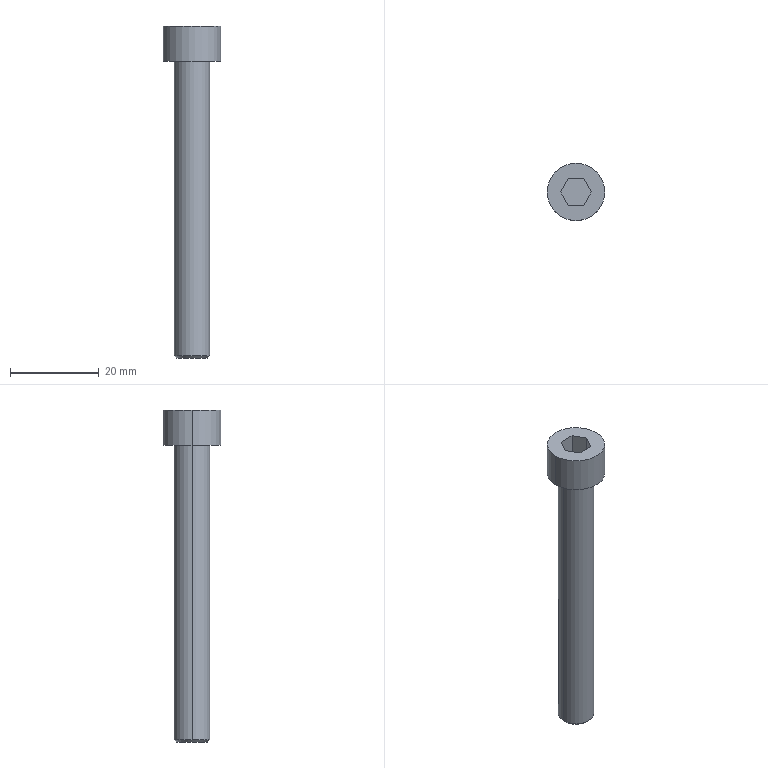Part | Creo | 1 solid | 16 faces | box 13 x 13 x 75 mm | volume 4262 mm3 | plane 10 | cylinder 4 | cone 2 | commonest cylinder face diameters 8 x2 13 x2
STEP:
#1=CARTESIAN_POINT('',(0.,0.,0.));
#2=DIRECTION('',(0.,0.,1.));
#3=DIRECTION('',(1.,0.,0.));
#4=AXIS2_PLACEMENT_3D('',#1,#2,#3);
#5=CARTESIAN_POINT('',(436.948,72.142,-161.289));
#6=VERTEX_POINT('',#5);
#7=CARTESIAN_POINT('',(444.948,72.142,-161.289));
#8=VERTEX_POINT('',#7);
#9=CARTESIAN_POINT('',(440.948,72.142,-161.289));
#10=DIRECTION('',(0.,0.,-1.));
#11=DIRECTION('',(-1.,0.,0.));
#12=AXIS2_PLACEMENT_3D('',#9,#10,#11);
#13=CIRCLE('',#12,4.);
#14=EDGE_CURVE('',#6,#8,#13,.T.);
#15=ORIENTED_EDGE('',*,*,#14,.T.);
#16=CARTESIAN_POINT('',(444.948,72.142,-94.796));
#17=VERTEX_POINT('',#16);
#18=CARTESIAN_POINT('',(444.948,72.142,-94.796));
#19=DIRECTION('',(0.,0.,-1.));
#20=VECTOR('',#19,66.493);
#21=LINE('',#18,#20);
#22=EDGE_CURVE('',#17,#8,#21,.T.);
#23=ORIENTED_EDGE('',*,*,#22,.F.);
#24=CARTESIAN_POINT('',(436.948,72.142,-94.796));
#25=VERTEX_POINT('',#24);
#26=CARTESIAN_POINT('',(440.948,72.142,-94.796));
#27=DIRECTION('',(0.,0.,1.));
#28=DIRECTION('',(1.,0.,0.));
#29=AXIS2_PLACEMENT_3D('',#26,#27,#28);
#30=CIRCLE('',#29,4.);
#31=EDGE_CURVE('',#17,#25,#30,.T.);
#32=ORIENTED_EDGE('',*,*,#31,.T.);
#33=CARTESIAN_POINT('',(436.948,72.142,-94.796));
#34=DIRECTION('',(0.,0.,-1.));
#35=VECTOR('',#34,66.493);
#36=LINE('',#33,#35);
#37=EDGE_CURVE('',#25,#6,#36,.T.);
#38=ORIENTED_EDGE('',*,*,#37,.T.);
#39=EDGE_LOOP('',(#15,#23,#32,#38));
#40=FACE_OUTER_BOUND('',#39,.F.);
#41=CARTESIAN_POINT('',(440.948,72.142,-94.796));
#42=DIRECTION('',(0.,0.,-1.));
#43=DIRECTION('',(-1.,0.,0.));
#44=AXIS2_PLACEMENT_3D('',#41,#42,#43);
#45=CYLINDRICAL_SURFACE('',#44,4.);
#46=ADVANCED_FACE('',(#40),#45,.T.);
#47=CARTESIAN_POINT('',(437.455,72.142,-161.796));
#48=VERTEX_POINT('',#47);
#49=CARTESIAN_POINT('',(444.441,72.142,-161.796));
#50=VERTEX_POINT('',#49);
#51=CARTESIAN_POINT('',(440.948,72.142,-161.796));
#52=DIRECTION('',(0.,0.,-1.));
#53=DIRECTION('',(-1.,0.,0.));
#54=AXIS2_PLACEMENT_3D('',#51,#52,#53);
#55=CIRCLE('',#54,3.493);
#56=EDGE_CURVE('',#48,#50,#55,.T.);
#57=ORIENTED_EDGE('',*,*,#56,.T.);
#58=CARTESIAN_POINT('',(444.441,72.142,-161.796));
#59=DIRECTION('',(0.7071,0.,0.7071));
#60=VECTOR('',#59,0.7176);
#61=LINE('',#58,#60);
#62=EDGE_CURVE('',#50,#8,#61,.T.);
#63=ORIENTED_EDGE('',*,*,#62,.T.);
#64=ORIENTED_EDGE('',*,*,#14,.F.);
#65=CARTESIAN_POINT('',(437.455,72.142,-161.796));
#66=DIRECTION('',(-0.7071,0.,0.7071));
#67=VECTOR('',#66,0.7176);
#68=LINE('',#65,#67);
#69=EDGE_CURVE('',#48,#6,#68,.T.);
#70=ORIENTED_EDGE('',*,*,#69,.F.);
#71=EDGE_LOOP('',(#57,#63,#64,#70));
#72=FACE_OUTER_BOUND('',#71,.F.);
#73=CARTESIAN_POINT('',(440.948,72.142,-161.543));
#74=DIRECTION('',(0.,0.,1.));
#75=DIRECTION('',(1.,0.,0.));
#76=AXIS2_PLACEMENT_3D('',#73,#74,#75);
#77=CONICAL_SURFACE('',#76,3.746,45.);
#78=ADVANCED_FACE('',(#72),#77,.T.);
#79=ORIENTED_EDGE('',*,*,#56,.F.);
#80=CARTESIAN_POINT('',(440.948,72.142,-161.796));
#81=DIRECTION('',(0.,0.,-1.));
#82=DIRECTION('',(1.,0.,0.));
#83=AXIS2_PLACEMENT_3D('',#80,#81,#82);
#84=CIRCLE('',#83,3.493);
#85=EDGE_CURVE('',#50,#48,#84,.T.);
#86=ORIENTED_EDGE('',*,*,#85,.F.);
#87=EDGE_LOOP('',(#79,#86));
#88=FACE_OUTER_BOUND('',#87,.F.);
#89=CARTESIAN_POINT('',(440.948,72.142,-161.796));
#90=DIRECTION('',(0.,0.,1.));
#91=DIRECTION('',(1.,0.,0.));
#92=AXIS2_PLACEMENT_3D('',#89,#90,#91);
#93=PLANE('',#92);
#94=ADVANCED_FACE('',(#88),#93,.F.);
#95=ORIENTED_EDGE('',*,*,#85,.T.);
#96=ORIENTED_EDGE('',*,*,#69,.T.);
#97=CARTESIAN_POINT('',(440.948,72.142,-161.289));
#98=DIRECTION('',(0.,0.,-1.));
#99=DIRECTION('',(1.,0.,0.));
#100=AXIS2_PLACEMENT_3D('',#97,#98,#99);
#101=CIRCLE('',#100,4.);
#102=EDGE_CURVE('',#8,#6,#101,.T.);
#103=ORIENTED_EDGE('',*,*,#102,.F.);
#104=ORIENTED_EDGE('',*,*,#62,.F.);
#105=EDGE_LOOP('',(#95,#96,#103,#104));
#106=FACE_OUTER_BOUND('',#105,.F.);
#107=CARTESIAN_POINT('',(440.948,72.142,-161.543));
#108=DIRECTION('',(0.,0.,1.));
#109=DIRECTION('',(1.,0.,0.));
#110=AXIS2_PLACEMENT_3D('',#107,#108,#109);
#111=CONICAL_SURFACE('',#110,3.746,45.);
#112=ADVANCED_FACE('',(#106),#111,.T.);
#113=ORIENTED_EDGE('',*,*,#102,.T.);
#114=ORIENTED_EDGE('',*,*,#37,.F.);
#115=CARTESIAN_POINT('',(440.948,72.142,-94.796));
#116=DIRECTION('',(0.,0.,1.));
#117=DIRECTION('',(-1.,0.,0.));
#118=AXIS2_PLACEMENT_3D('',#115,#116,#117);
#119=CIRCLE('',#118,4.);
#120=EDGE_CURVE('',#25,#17,#119,.T.);
#121=ORIENTED_EDGE('',*,*,#120,.T.);
#122=ORIENTED_EDGE('',*,*,#22,.T.);
#123=EDGE_LOOP('',(#113,#114,#121,#122));
#124=FACE_OUTER_BOUND('',#123,.F.);
#125=CARTESIAN_POINT('',(440.948,72.142,-94.796));
#126=DIRECTION('',(0.,0.,-1.));
#127=DIRECTION('',(-1.,0.,0.));
#128=AXIS2_PLACEMENT_3D('',#125,#126,#127);
#129=CYLINDRICAL_SURFACE('',#128,4.);
#130=ADVANCED_FACE('',(#124),#129,.T.);
#131=CARTESIAN_POINT('',(434.448,72.142,-94.796));
#132=VERTEX_POINT('',#131);
#133=CARTESIAN_POINT('',(447.448,72.142,-94.796));
#134=VERTEX_POINT('',#133);
#135=CARTESIAN_POINT('',(440.948,72.142,-94.796));
#136=DIRECTION('',(0.,0.,-1.));
#137=DIRECTION('',(-1.,0.,0.));
#138=AXIS2_PLACEMENT_3D('',#135,#136,#137);
#139=CIRCLE('',#138,6.5);
#140=EDGE_CURVE('',#132,#134,#139,.T.);
#141=ORIENTED_EDGE('',*,*,#140,.F.);
#142=CARTESIAN_POINT('',(440.948,72.142,-94.796));
#143=DIRECTION('',(0.,0.,-1.));
#144=DIRECTION('',(1.,0.,0.));
#145=AXIS2_PLACEMENT_3D('',#142,#143,#144);
#146=CIRCLE('',#145,6.5);
#147=EDGE_CURVE('',#134,#132,#146,.T.);
#148=ORIENTED_EDGE('',*,*,#147,.F.);
#149=EDGE_LOOP('',(#141,#148));
#150=FACE_OUTER_BOUND('',#149,.F.);
#151=ORIENTED_EDGE('',*,*,#120,.F.);
#152=ORIENTED_EDGE('',*,*,#31,.F.);
#153=EDGE_LOOP('',(#151,#152));
#154=FACE_BOUND('',#153,.F.);
#155=CARTESIAN_POINT('',(440.948,72.142,-94.796));
#156=DIRECTION('',(0.,0.,-1.));
#157=DIRECTION('',(-1.,0.,0.));
#158=AXIS2_PLACEMENT_3D('',#155,#156,#157);
#159=PLANE('',#158);
#160=ADVANCED_FACE('',(#150,#154),#159,.T.);
#161=CARTESIAN_POINT('',(447.448,72.142,-86.796));
#162=VERTEX_POINT('',#161);
#163=CARTESIAN_POINT('',(434.448,72.142,-86.796));
#164=VERTEX_POINT('',#163);
#165=CARTESIAN_POINT('',(440.948,72.142,-86.796));
#166=DIRECTION('',(0.,0.,1.));
#167=DIRECTION('',(1.,0.,0.));
#168=AXIS2_PLACEMENT_3D('',#165,#166,#167);
#169=CIRCLE('',#168,6.5);
#170=EDGE_CURVE('',#162,#164,#169,.T.);
#171=ORIENTED_EDGE('',*,*,#170,.T.);
#172=CARTESIAN_POINT('',(434.448,72.142,-94.796));
#173=DIRECTION('',(0.,0.,1.));
#174=VECTOR('',#173,8.);
#175=LINE('',#172,#174);
#176=EDGE_CURVE('',#132,#164,#175,.T.);
#177=ORIENTED_EDGE('',*,*,#176,.F.);
#178=ORIENTED_EDGE('',*,*,#140,.T.);
#179=CARTESIAN_POINT('',(447.448,72.142,-94.796));
#180=DIRECTION('',(0.,0.,1.));
#181=VECTOR('',#180,8.);
#182=LINE('',#179,#181);
#183=EDGE_CURVE('',#134,#162,#182,.T.);
#184=ORIENTED_EDGE('',*,*,#183,.T.);
#185=EDGE_LOOP('',(#171,#177,#178,#184));
#186=FACE_OUTER_BOUND('',#185,.F.);
#187=CARTESIAN_POINT('',(440.948,72.142,-94.796));
#188=DIRECTION('',(0.,0.,1.));
#189=DIRECTION('',(1.,0.,0.));
#190=AXIS2_PLACEMENT_3D('',#187,#188,#189);
#191=CYLINDRICAL_SURFACE('',#190,6.5);
#192=ADVANCED_FACE('',(#186),#191,.T.);
#193=CARTESIAN_POINT('',(440.948,72.142,-86.796));
#194=DIRECTION('',(0.,0.,1.));
#195=DIRECTION('',(-1.,0.,0.));
#196=AXIS2_PLACEMENT_3D('',#193,#194,#195);
#197=CIRCLE('',#196,6.5);
#198=EDGE_CURVE('',#164,#162,#197,.T.);
#199=ORIENTED_EDGE('',*,*,#198,.F.);
#200=ORIENTED_EDGE('',*,*,#170,.F.);
#201=EDGE_LOOP('',(#199,#200));
#202=FACE_OUTER_BOUND('',#201,.F.);
#203=CARTESIAN_POINT('',(439.216,75.142,-86.796));
#204=VERTEX_POINT('',#203);
#205=CARTESIAN_POINT('',(442.68,75.142,-86.796));
#206=VERTEX_POINT('',#205);
#207=CARTESIAN_POINT('',(439.216,75.142,-86.796));
#208=DIRECTION('',(1.,0.,0.));
#209=VECTOR('',#208,3.464);
#210=LINE('',#207,#209);
#211=EDGE_CURVE('',#204,#206,#210,.T.);
#212=ORIENTED_EDGE('',*,*,#211,.F.);
#213=CARTESIAN_POINT('',(437.484,72.142,-86.796));
#214=VERTEX_POINT('',#213);
#215=CARTESIAN_POINT('',(437.484,72.142,-86.796));
#216=DIRECTION('',(0.5,0.866,0.));
#217=VECTOR('',#216,3.464);
#218=LINE('',#215,#217);
#219=EDGE_CURVE('',#214,#204,#218,.T.);
#220=ORIENTED_EDGE('',*,*,#219,.F.);
#221=CARTESIAN_POINT('',(439.216,69.142,-86.796));
#222=VERTEX_POINT('',#221);
#223=CARTESIAN_POINT('',(439.216,69.142,-86.796));
#224=DIRECTION('',(-0.5,0.866,0.));
#225=VECTOR('',#224,3.464);
#226=LINE('',#223,#225);
#227=EDGE_CURVE('',#222,#214,#226,.T.);
#228=ORIENTED_EDGE('',*,*,#227,.F.);
#229=CARTESIAN_POINT('',(442.68,69.142,-86.796));
#230=VERTEX_POINT('',#229);
#231=CARTESIAN_POINT('',(442.68,69.142,-86.796));
#232=DIRECTION('',(-1.,0.,0.));
#233=VECTOR('',#232,3.464);
#234=LINE('',#231,#233);
#235=EDGE_CURVE('',#230,#222,#234,.T.);
#236=ORIENTED_EDGE('',*,*,#235,.F.);
#237=CARTESIAN_POINT('',(444.412,72.142,-86.796));
#238=VERTEX_POINT('',#237);
#239=CARTESIAN_POINT('',(444.412,72.142,-86.796));
#240=DIRECTION('',(-0.5,-0.866,0.));
#241=VECTOR('',#240,3.464);
#242=LINE('',#239,#241);
#243=EDGE_CURVE('',#238,#230,#242,.T.);
#244=ORIENTED_EDGE('',*,*,#243,.F.);
#245=CARTESIAN_POINT('',(442.68,75.142,-86.796));
#246=DIRECTION('',(0.5,-0.866,0.));
#247=VECTOR('',#246,3.464);
#248=LINE('',#245,#247);
#249=EDGE_CURVE('',#206,#238,#248,.T.);
#250=ORIENTED_EDGE('',*,*,#249,.F.);
#251=EDGE_LOOP('',(#212,#220,#228,#236,#244,#250));
#252=FACE_BOUND('',#251,.F.);
#253=CARTESIAN_POINT('',(440.948,72.142,-86.796));
#254=DIRECTION('',(0.,0.,1.));
#255=DIRECTION('',(1.,0.,0.));
#256=AXIS2_PLACEMENT_3D('',#253,#254,#255);
#257=PLANE('',#256);
#258=ADVANCED_FACE('',(#202,#252),#257,.T.);
#259=ORIENTED_EDGE('',*,*,#211,.T.);
#260=CARTESIAN_POINT('',(442.68,75.142,-92.076));
#261=VERTEX_POINT('',#260);
#262=CARTESIAN_POINT('',(442.68,75.142,-86.796));
#263=DIRECTION('',(0.,0.,-1.));
#264=VECTOR('',#263,5.28);
#265=LINE('',#262,#264);
#266=EDGE_CURVE('',#206,#261,#265,.T.);
#267=ORIENTED_EDGE('',*,*,#266,.T.);
#268=CARTESIAN_POINT('',(439.216,75.142,-92.076));
#269=VERTEX_POINT('',#268);
#270=CARTESIAN_POINT('',(439.216,75.142,-92.076));
#271=DIRECTION('',(1.,0.,0.));
#272=VECTOR('',#271,3.464);
#273=LINE('',#270,#272);
#274=EDGE_CURVE('',#269,#261,#273,.T.);
#275=ORIENTED_EDGE('',*,*,#274,.F.);
#276=CARTESIAN_POINT('',(439.216,75.142,-86.796));
#277=DIRECTION('',(0.,0.,-1.));
#278=VECTOR('',#277,5.28);
#279=LINE('',#276,#278);
#280=EDGE_CURVE('',#204,#269,#279,.T.);
#281=ORIENTED_EDGE('',*,*,#280,.F.);
#282=EDGE_LOOP('',(#259,#267,#275,#281));
#283=FACE_OUTER_BOUND('',#282,.F.);
#284=CARTESIAN_POINT('',(442.68,75.142,-92.076));
#285=DIRECTION('',(0.,1.,0.));
#286=DIRECTION('',(0.,0.,1.));
#287=AXIS2_PLACEMENT_3D('',#284,#285,#286);
#288=PLANE('',#287);
#289=ADVANCED_FACE('',(#283),#288,.F.);
#290=ORIENTED_EDGE('',*,*,#249,.T.);
#291=CARTESIAN_POINT('',(444.412,72.142,-92.076));
#292=VERTEX_POINT('',#291);
#293=CARTESIAN_POINT('',(444.412,72.142,-86.796));
#294=DIRECTION('',(0.,0.,-1.));
#295=VECTOR('',#294,5.28);
#296=LINE('',#293,#295);
#297=EDGE_CURVE('',#238,#292,#296,.T.);
#298=ORIENTED_EDGE('',*,*,#297,.T.);
#299=CARTESIAN_POINT('',(444.412,72.142,-92.076));
#300=DIRECTION('',(-0.5,0.866,0.));
#301=VECTOR('',#300,3.464);
#302=LINE('',#299,#301);
#303=EDGE_CURVE('',#292,#261,#302,.T.);
#304=ORIENTED_EDGE('',*,*,#303,.T.);
#305=ORIENTED_EDGE('',*,*,#266,.F.);
#306=EDGE_LOOP('',(#290,#298,#304,#305));
#307=FACE_OUTER_BOUND('',#306,.F.);
#308=CARTESIAN_POINT('',(444.412,72.142,-92.076));
#309=DIRECTION('',(0.866,0.5,0.));
#310=DIRECTION('',(-0.5,0.866,0.));
#311=AXIS2_PLACEMENT_3D('',#308,#309,#310);
#312=PLANE('',#311);
#313=ADVANCED_FACE('',(#307),#312,.F.);
#314=ORIENTED_EDGE('',*,*,#243,.T.);
#315=CARTESIAN_POINT('',(442.68,69.142,-92.076));
#316=VERTEX_POINT('',#315);
#317=CARTESIAN_POINT('',(442.68,69.142,-86.796));
#318=DIRECTION('',(0.,0.,-1.));
#319=VECTOR('',#318,5.28);
#320=LINE('',#317,#319);
#321=EDGE_CURVE('',#230,#316,#320,.T.);
#322=ORIENTED_EDGE('',*,*,#321,.T.);
#323=CARTESIAN_POINT('',(442.68,69.142,-92.076));
#324=DIRECTION('',(0.5,0.866,0.));
#325=VECTOR('',#324,3.464);
#326=LINE('',#323,#325);
#327=EDGE_CURVE('',#316,#292,#326,.T.);
#328=ORIENTED_EDGE('',*,*,#327,.T.);
#329=ORIENTED_EDGE('',*,*,#297,.F.);
#330=EDGE_LOOP('',(#314,#322,#328,#329));
#331=FACE_OUTER_BOUND('',#330,.F.);
#332=CARTESIAN_POINT('',(442.68,69.142,-92.076));
#333=DIRECTION('',(0.866,-0.5,0.));
#334=DIRECTION('',(0.5,0.866,0.));
#335=AXIS2_PLACEMENT_3D('',#332,#333,#334);
#336=PLANE('',#335);
#337=ADVANCED_FACE('',(#331),#336,.F.);
#338=ORIENTED_EDGE('',*,*,#235,.T.);
#339=CARTESIAN_POINT('',(439.216,69.142,-92.076));
#340=VERTEX_POINT('',#339);
#341=CARTESIAN_POINT('',(439.216,69.142,-86.796));
#342=DIRECTION('',(0.,0.,-1.));
#343=VECTOR('',#342,5.28);
#344=LINE('',#341,#343);
#345=EDGE_CURVE('',#222,#340,#344,.T.);
#346=ORIENTED_EDGE('',*,*,#345,.T.);
#347=CARTESIAN_POINT('',(442.68,69.142,-92.076));
#348=DIRECTION('',(-1.,0.,0.));
#349=VECTOR('',#348,3.464);
#350=LINE('',#347,#349);
#351=EDGE_CURVE('',#316,#340,#350,.T.);
#352=ORIENTED_EDGE('',*,*,#351,.F.);
#353=ORIENTED_EDGE('',*,*,#321,.F.);
#354=EDGE_LOOP('',(#338,#346,#352,#353));
#355=FACE_OUTER_BOUND('',#354,.F.);
#356=CARTESIAN_POINT('',(439.216,69.142,-92.076));
#357=DIRECTION('',(0.,-1.,0.));
#358=DIRECTION('',(0.,0.,-1.));
#359=AXIS2_PLACEMENT_3D('',#356,#357,#358);
#360=PLANE('',#359);
#361=ADVANCED_FACE('',(#355),#360,.F.);
#362=ORIENTED_EDGE('',*,*,#227,.T.);
#363=CARTESIAN_POINT('',(437.484,72.142,-92.076));
#364=VERTEX_POINT('',#363);
#365=CARTESIAN_POINT('',(437.484,72.142,-86.796));
#366=DIRECTION('',(0.,0.,-1.));
#367=VECTOR('',#366,5.28);
#368=LINE('',#365,#367);
#369=EDGE_CURVE('',#214,#364,#368,.T.);
#370=ORIENTED_EDGE('',*,*,#369,.T.);
#371=CARTESIAN_POINT('',(437.484,72.142,-92.076));
#372=DIRECTION('',(0.5,-0.866,0.));
#373=VECTOR('',#372,3.464);
#374=LINE('',#371,#373);
#375=EDGE_CURVE('',#364,#340,#374,.T.);
#376=ORIENTED_EDGE('',*,*,#375,.T.);
#377=ORIENTED_EDGE('',*,*,#345,.F.);
#378=EDGE_LOOP('',(#362,#370,#376,#377));
#379=FACE_OUTER_BOUND('',#378,.F.);
#380=CARTESIAN_POINT('',(437.484,72.142,-92.076));
#381=DIRECTION('',(-0.866,-0.5,0.));
#382=DIRECTION('',(0.5,-0.866,0.));
#383=AXIS2_PLACEMENT_3D('',#380,#381,#382);
#384=PLANE('',#383);
#385=ADVANCED_FACE('',(#379),#384,.F.);
#386=ORIENTED_EDGE('',*,*,#219,.T.);
#387=ORIENTED_EDGE('',*,*,#280,.T.);
#388=CARTESIAN_POINT('',(439.216,75.142,-92.076));
#389=DIRECTION('',(-0.5,-0.866,0.));
#390=VECTOR('',#389,3.464);
#391=LINE('',#388,#390);
#392=EDGE_CURVE('',#269,#364,#391,.T.);
#393=ORIENTED_EDGE('',*,*,#392,.T.);
#394=ORIENTED_EDGE('',*,*,#369,.F.);
#395=EDGE_LOOP('',(#386,#387,#393,#394));
#396=FACE_OUTER_BOUND('',#395,.F.);
#397=CARTESIAN_POINT('',(439.216,75.142,-92.076));
#398=DIRECTION('',(-0.866,0.5,0.));
#399=DIRECTION('',(-0.5,-0.866,0.));
#400=AXIS2_PLACEMENT_3D('',#397,#398,#399);
#401=PLANE('',#400);
#402=ADVANCED_FACE('',(#396),#401,.F.);
#403=ORIENTED_EDGE('',*,*,#274,.T.);
#404=ORIENTED_EDGE('',*,*,#303,.F.);
#405=ORIENTED_EDGE('',*,*,#327,.F.);
#406=ORIENTED_EDGE('',*,*,#351,.T.);
#407=ORIENTED_EDGE('',*,*,#375,.F.);
#408=ORIENTED_EDGE('',*,*,#392,.F.);
#409=EDGE_LOOP('',(#403,#404,#405,#406,#407,#408));
#410=FACE_OUTER_BOUND('',#409,.F.);
#411=CARTESIAN_POINT('',(439.216,75.142,-92.076));
#412=DIRECTION('',(0.,0.,1.));
#413=DIRECTION('',(1.,0.,0.));
#414=AXIS2_PLACEMENT_3D('',#411,#412,#413);
#415=PLANE('',#414);
#416=ADVANCED_FACE('',(#410),#415,.T.);
#417=ORIENTED_EDGE('',*,*,#198,.T.);
#418=ORIENTED_EDGE('',*,*,#183,.F.);
#419=ORIENTED_EDGE('',*,*,#147,.T.);
#420=ORIENTED_EDGE('',*,*,#176,.T.);
#421=EDGE_LOOP('',(#417,#418,#419,#420));
#422=FACE_OUTER_BOUND('',#421,.F.);
#423=CARTESIAN_POINT('',(440.948,72.142,-94.796));
#424=DIRECTION('',(0.,0.,1.));
#425=DIRECTION('',(1.,0.,0.));
#426=AXIS2_PLACEMENT_3D('',#423,#424,#425);
#427=CYLINDRICAL_SURFACE('',#426,6.5);
#428=ADVANCED_FACE('',(#422),#427,.T.);
#429=CLOSED_SHELL('',(#46,#78,#94,#112,#130,#160,#192,#258,#289,#313,#337,#361,#385,#402,#416,#428));
#430=MANIFOLD_SOLID_BREP('',#429);
#431=(LENGTH_UNIT()NAMED_UNIT(*)SI_UNIT(.MILLI.,.METRE.));
#432=UNCERTAINTY_MEASURE_WITH_UNIT(LENGTH_MEASURE(0.007722),#431,'','');
#433=(NAMED_UNIT(*)PLANE_ANGLE_UNIT()SI_UNIT($,.RADIAN.));
#434=PLANE_ANGLE_MEASURE_WITH_UNIT(PLANE_ANGLE_MEASURE(0.01745),#433);
#435=(CONVERSION_BASED_UNIT('DEGREE',#434)NAMED_UNIT(*)PLANE_ANGLE_UNIT());
#436=(NAMED_UNIT(*)SI_UNIT($,.STERADIAN.)SOLID_ANGLE_UNIT());
#437=(GEOMETRIC_REPRESENTATION_CONTEXT(3)GLOBAL_UNCERTAINTY_ASSIGNED_CONTEXT((#432))GLOBAL_UNIT_ASSIGNED_CONTEXT((#431,#435,#436))REPRESENTATION_CONTEXT('',''));
#438=ADVANCED_BREP_SHAPE_REPRESENTATION('',(#4,#430),#437);